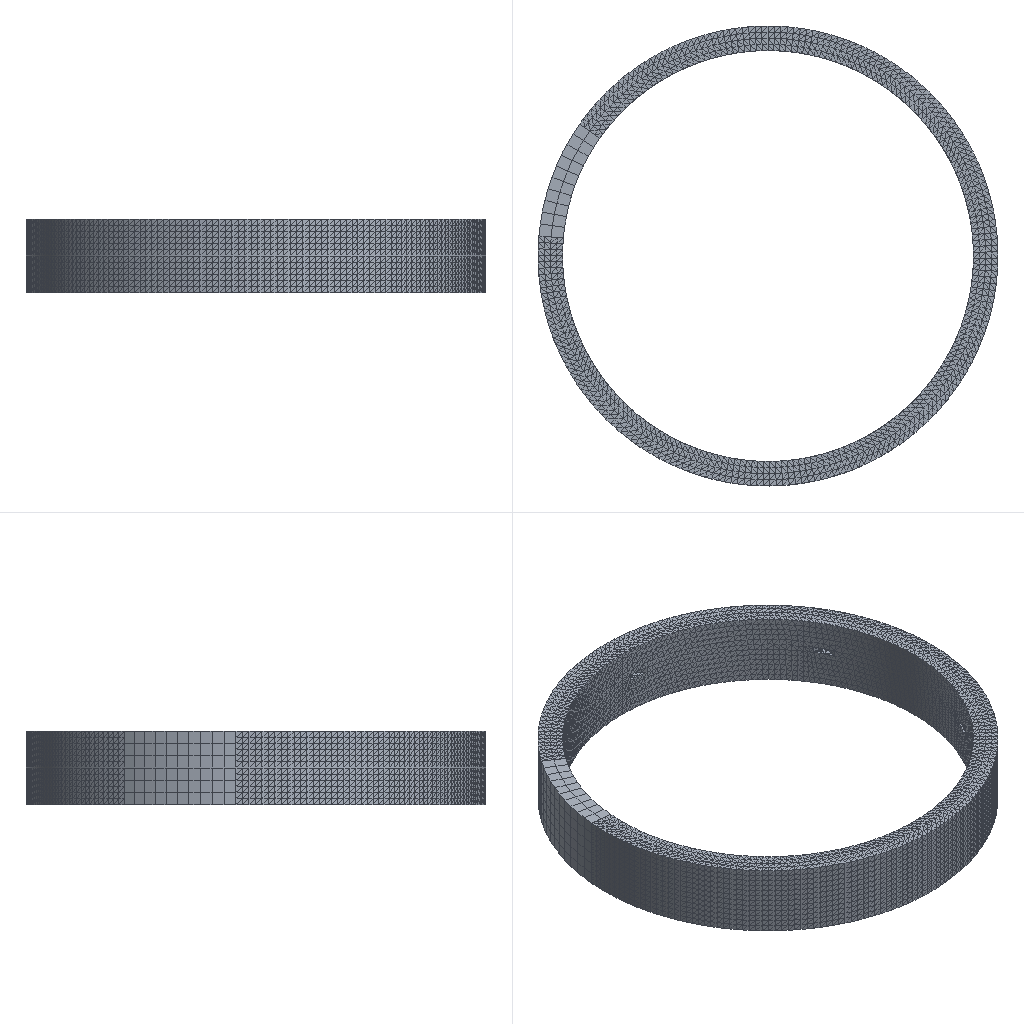Simulation study | abaqus
Set-up summary:
category,name,step,type,value,unit,region
solver,abaqus
solver,version,,,Abaqus/Standard 2020
units,not stated in the deck,,not stated
analysis,deck,,static,static
load_step,Step-1,Step-1,static
load_step,requested,,,1
mesh,nodes,,,120599
mesh,elements,,,97952
element_type,C3D4,,solid,24332
element_type,C3D10,,solid,73500
element_type,C3D8R,,solid,120
load,load commands in deck,,count,2
bc,support commands in deck,,count,1
material,GUANPIAN,,in results
material,LUOSHUAN,,in results
check,setup vs results,,match,"per instance, exact: element labels, types and connectivity; labels of the nodes the elements use; coordinates not compared"
Abaqus input file, long lists of numbers shortened, first 334 of 1919 lines:
*Heading
** Job name: Job-1 Model name: Model-1
** Generated by: Abaqus/CAE 2020
*Preprint, echo=NO, model=NO, history=NO, contact=NO
**
** PARTS
**
*Part, name=Part-1
*Node
      1,   5415.547,    6910.075,         600.
      2,   2137.132,    6910.075,         600.
** (18888 more lines like these left out)
*Element, type=C3D10
   1, 1664,  747, 1665, 1666, 2706, 2705, 2704, 2708, 2707, 2709
   2, 1667, 1666, 1665,  531, 2711, 2709, 2710, 2713, 2712, 2714
** (12248 more lines like these left out)
*Nset, nset=Set-33, generate
     1,  18890,      1
*Elset, elset=Set-33, generate
     1,  12250,      1
** Section: Section-1
*Solid Section, elset=Set-33, material=guanpian
,
*End Part
**
*Part, name=huan
*Node
      1,        -737.,   3267.925,        1200.
      2,  -907.02,   3224.875,        1200.
** (229 more lines like these left out)
*Element, type=C3D8R
  1,  78,  79,  90,  89,   1,   2,  13,  12
  2,  79,  80,  91,  90,   2,   3,  14,  13
** (118 more lines like these left out)
*Nset, nset=Set-1, generate
   1,  231,    1
*Elset, elset=Set-1, generate
   1,  120,    1
** Section: Section-1
*Solid Section, elset=Set-1, material=guanpian
,
*End Part
**
*Part, name=luoshuan
*Node
      1,   1815.458,  -103.665,   603.43
      2,   1794.725,  -75.309,    565.088
** (1002 more lines like these left out)
*Element, type=C3D4
  1, 842, 843, 844, 845
  2, 842, 846,  47,   7
** (3474 more lines like these left out)
*Nset, nset=Set-3, generate
    1,  1004,     1
*Elset, elset=Set-3, generate
    1,  3476,     1
** Section: Section-2
*Solid Section, elset=Set-3, material=luoshuan
,
*End Part
**
**
** ASSEMBLY
**
*Assembly, name=Assembly
**
*Instance, name=luoshuan-1, part=luoshuan
2639.383, 121.344, -1266.961
2639.383, 121.344, -1266.961, 2640.007, 121.614, -1266.228, 146.146
*End Instance
**
*Instance, name=Part-1-2, part=Part-1
4357.09, -7001.414,         600.
4357.09, -7001.414,         600., 4357.328, -7000.443,         600.,         180.
*End Instance
**
*Instance, name=luoshuan-1-rad-2, part=luoshuan
4357.446, -663.937, -1266.961
4357.446, -663.937, -1266.961, 4358.245, -663.994, -1266.362, 108.805
*End Instance
**
*Instance, name=luoshuan-1-rad-3, part=luoshuan
4699.623, -2521.711, -1266.961
4699.623, -2521.711, -1266.961, 4700.449, -2522.219, -1266.717, 84.284
*End Instance
**
*Instance, name=luoshuan-1-rad-4, part=luoshuan
3374.088, -3867.581, -1266.961
3374.088, -3867.581, -1266.961, 3374.579, -3868.402, -1267.251, 85.669
*End Instance
**
*Instance, name=Part-1-2-rad-2, part=Part-1
-491.939, -6156.447,         600.
-491.939, -6156.447,         600., -491.28, -6155.695,         600.,         180.
*End Instance
**
*Instance, name=Part-1-2-rad-3, part=Part-1
-2581.071, -1699.701,         600.
-2581.071, -1699.701,         600., -2580.139, -1699.339,         600.,         180.
*End Instance
**
*Instance, name=Part-1-2-rad-4, part=Part-1
-128.596, 2567.9,         600.
-128.596, 2567.9,         600., -127.602, 2567.791,         600.,         180.
*End Instance
**
*Instance, name=luoshuan-1-rad-2-1, part=luoshuan
1010.677, -835.593, -1266.961
1010.677, -835.593, -1266.961, 1011.089, -835.087, -1266.203, 187.52
*End Instance
**
*Instance, name=luoshuan-1-rad-3-1, part=luoshuan
698.5, -1799.706, -1266.961
698.5, -1799.706, -1266.961, 698.765, -1799.084, -1266.225, 211.514
*End Instance
**
*Instance, name=Part-1-2-rad-2-1, part=Part-1
7830.536, -3513.975,         600.
7830.536, -3513.975,         600., 7830.298, -3513.004,         600.,         180.
*End Instance
**
*Instance, name=luoshuan-1-rad-3-1-rad-2, part=luoshuan
1511.32, -3553.725, -1266.961
1511.32, -3553.725, -1266.961, 1511.366, -3554.509, -1267.581, 111.965
*End Instance
**
*Instance, name=Part-1-2-rad-3-1-rad-2, part=Part-1
4773.9, 3006.745,         600.
4773.9, 3006.745,         600., 4774.732, 3006.19,         600.,         180.
*End Instance
**
*Instance, name=huan-1, part=huan
2744.211, -1920.892,        -600.
2744.211, -1920.892,        -600., 2744.211, -1920.892, -599., 42.3
*End Instance
**
*Node
      1,   2744.159,  -1921.481,           0.
*Nset, nset=Set-5, instance=Part-1-2
     1,     4,     7,     8,    27,    28,    29,    30,   104,   105,   106,   107,   108,   149,   150,   151
   152,   153,   154,   155,   294,   300,   301,   302,   303,   304,   305,   306,   307,   308,   309,   310
** (24 more lines like these left out)
*Nset, nset=Set-5, instance=Part-1-2-rad-2
     1,     4,     7,     8,    27,    28,    29,    30,   104,   105,   106,   107,   108,   149,   150,   151
   152,   153,   154,   155,   294,   300,   301,   302,   303,   304,   305,   306,   307,   308,   309,   310
** (24 more lines like these left out)
*Nset, nset=Set-5, instance=Part-1-2-rad-3
     1,     4,     7,     8,    27,    28,    29,    30,   104,   105,   106,   107,   108,   149,   150,   151
   152,   153,   154,   155,   294,   300,   301,   302,   303,   304,   305,   306,   307,   308,   309,   310
** (24 more lines like these left out)
*Nset, nset=Set-5, instance=Part-1-2-rad-2-1
     1,     4,     7,     8,    27,    28,    29,    30,   104,   105,   106,   107,   108,   149,   150,   151
   152,   153,   154,   155,   294,   300,   301,   302,   303,   304,   305,   306,   307,   308,   309,   310
** (24 more lines like these left out)
*Nset, nset=Set-5, instance=Part-1-2-rad-4
     1,     4,     7,     8,    27,    28,    29,    30,   104,   105,   106,   107,   108,   149,   150,   151
   152,   153,   154,   155,   294,   300,   301,   302,   303,   304,   305,   306,   307,   308,   309,   310
** (24 more lines like these left out)
*Nset, nset=Set-5, instance=huan-1
  67,  68,  69,  70,  71,  72,  73,  74,  75,  76,  77, 144, 145, 146, 147, 148
 149, 150, 151, 152, 153, 154, 221, 222, 223, 224, 225, 226, 227, 228, 229, 230
** (1 more lines like these left out)
*Nset, nset=Set-5, instance=Part-1-2-rad-3-1-rad-2
     1,     4,     7,     8,    27,    28,    29,    30,   104,   105,   106,   107,   108,   149,   150,   151
   152,   153,   154,   155,   294,   300,   301,   302,   303,   304,   305,   306,   307,   308,   309,   310
** (24 more lines like these left out)
*Elset, elset=Set-5, instance=Part-1-2
  558,  646,  843, 1385, 1387, 1492, 1602, 1660, 1726, 1870, 2208, 2224, 2319, 2323, 2374, 2393
 2559, 2567, 2753, 2761, 2774, 2784, 2785, 2788, 6117, 6127, 6128, 6132, 6134, 6177, 6178, 6181
** (8 more lines like these left out)
*Elset, elset=Set-5, instance=Part-1-2-rad-2
  558,  646,  843, 1385, 1387, 1492, 1602, 1660, 1726, 1870, 2208, 2224, 2319, 2323, 2374, 2393
 2559, 2567, 2753, 2761, 2774, 2784, 2785, 2788, 6117, 6127, 6128, 6132, 6134, 6177, 6178, 6181
** (8 more lines like these left out)
*Elset, elset=Set-5, instance=Part-1-2-rad-3
  558,  646,  843, 1385, 1387, 1492, 1602, 1660, 1726, 1870, 2208, 2224, 2319, 2323, 2374, 2393
 2559, 2567, 2753, 2761, 2774, 2784, 2785, 2788, 6117, 6127, 6128, 6132, 6134, 6177, 6178, 6181
** (8 more lines like these left out)
*Elset, elset=Set-5, instance=Part-1-2-rad-2-1
  558,  646,  843, 1385, 1387, 1492, 1602, 1660, 1726, 1870, 2208, 2224, 2319, 2323, 2374, 2393
 2559, 2567, 2753, 2761, 2774, 2784, 2785, 2788, 6117, 6127, 6128, 6132, 6134, 6177, 6178, 6181
** (8 more lines like these left out)
*Elset, elset=Set-5, instance=Part-1-2-rad-4
  558,  646,  843, 1385, 1387, 1492, 1602, 1660, 1726, 1870, 2208, 2224, 2319, 2323, 2374, 2393
 2559, 2567, 2753, 2761, 2774, 2784, 2785, 2788, 6117, 6127, 6128, 6132, 6134, 6177, 6178, 6181
** (8 more lines like these left out)
*Elset, elset=Set-5, instance=huan-1
  51,  52,  53,  54,  55,  56,  57,  58,  59,  60, 111, 112, 113, 114, 115, 116
 117, 118, 119, 120
*Elset, elset=Set-5, instance=Part-1-2-rad-3-1-rad-2
  558,  646,  843, 1385, 1387, 1492, 1602, 1660, 1726, 1870, 2208, 2224, 2319, 2323, 2374, 2393
 2559, 2567, 2753, 2761, 2774, 2784, 2785, 2788, 6117, 6127, 6128, 6132, 6134, 6177, 6178, 6181
** (8 more lines like these left out)
*Nset, nset=Set-7
 1,
*Nset, nset=Set-8
 1,
*Nset, nset=Set-9, instance=Part-1-2
     1,     4,     7,     8,    27,    28,    29,    30,   104,   105,   106,   107,   108,   149,   150,   151
   152,   153,   154,   155,   294,   300,   301,   302,   303,   304,   305,   306,   307,   308,   309,   310
** (24 more lines like these left out)
*Nset, nset=Set-9, instance=Part-1-2-rad-2
     1,     4,     7,     8,    27,    28,    29,    30,   104,   105,   106,   107,   108,   149,   150,   151
   152,   153,   154,   155,   294,   300,   301,   302,   303,   304,   305,   306,   307,   308,   309,   310
** (24 more lines like these left out)
*Nset, nset=Set-9, instance=Part-1-2-rad-3
     1,     4,     7,     8,    27,    28,    29,    30,   104,   105,   106,   107,   108,   149,   150,   151
   152,   153,   154,   155,   294,   300,   301,   302,   303,   304,   305,   306,   307,   308,   309,   310
** (24 more lines like these left out)
*Nset, nset=Set-9, instance=Part-1-2-rad-2-1
     1,     4,     7,     8,    27,    28,    29,    30,   104,   105,   106,   107,   108,   149,   150,   151
   152,   153,   154,   155,   294,   300,   301,   302,   303,   304,   305,   306,   307,   308,   309,   310
** (24 more lines like these left out)
*Nset, nset=Set-9, instance=Part-1-2-rad-4
     1,     4,     7,     8,    27,    28,    29,    30,   104,   105,   106,   107,   108,   149,   150,   151
   152,   153,   154,   155,   294,   300,   301,   302,   303,   304,   305,   306,   307,   308,   309,   310
** (24 more lines like these left out)
*Nset, nset=Set-9, instance=Part-1-2-rad-3-1-rad-2
     1,     4,     7,     8,    27,    28,    29,    30,   104,   105,   106,   107,   108,   149,   150,   151
   152,   153,   154,   155,   294,   300,   301,   302,   303,   304,   305,   306,   307,   308,   309,   310
** (24 more lines like these left out)
*Elset, elset=Set-9, instance=Part-1-2
  558,  646,  843, 1385, 1387, 1492, 1602, 1660, 1726, 1870, 2208, 2224, 2319, 2323, 2374, 2393
 2559, 2567, 2753, 2761, 2774, 2784, 2785, 2788, 6117, 6127, 6128, 6132, 6134, 6177, 6178, 6181
** (8 more lines like these left out)
*Elset, elset=Set-9, instance=Part-1-2-rad-2
  558,  646,  843, 1385, 1387, 1492, 1602, 1660, 1726, 1870, 2208, 2224, 2319, 2323, 2374, 2393
 2559, 2567, 2753, 2761, 2774, 2784, 2785, 2788, 6117, 6127, 6128, 6132, 6134, 6177, 6178, 6181
** (8 more lines like these left out)
*Elset, elset=Set-9, instance=Part-1-2-rad-3
  558,  646,  843, 1385, 1387, 1492, 1602, 1660, 1726, 1870, 2208, 2224, 2319, 2323, 2374, 2393
 2559, 2567, 2753, 2761, 2774, 2784, 2785, 2788, 6117, 6127, 6128, 6132, 6134, 6177, 6178, 6181
** (8 more lines like these left out)
*Elset, elset=Set-9, instance=Part-1-2-rad-2-1
  558,  646,  843, 1385, 1387, 1492, 1602, 1660, 1726, 1870, 2208, 2224, 2319, 2323, 2374, 2393
 2559, 2567, 2753, 2761, 2774, 2784, 2785, 2788, 6117, 6127, 6128, 6132, 6134, 6177, 6178, 6181
** (8 more lines like these left out)
*Elset, elset=Set-9, instance=Part-1-2-rad-4
  558,  646,  843, 1385, 1387, 1492, 1602, 1660, 1726, 1870, 2208, 2224, 2319, 2323, 2374, 2393
 2559, 2567, 2753, 2761, 2774, 2784, 2785, 2788, 6117, 6127, 6128, 6132, 6134, 6177, 6178, 6181
** (8 more lines like these left out)
*Elset, elset=Set-9, instance=Part-1-2-rad-3-1-rad-2
  558,  646,  843, 1385, 1387, 1492, 1602, 1660, 1726, 1870, 2208, 2224, 2319, 2323, 2374, 2393
 2559, 2567, 2753, 2761, 2774, 2784, 2785, 2788, 6117, 6127, 6128, 6132, 6134, 6177, 6178, 6181
** (8 more lines like these left out)
*Nset, nset=m_Set-6, instance=luoshuan-1, generate
    1,  1004,     1
*Nset, nset=m_Set-6, instance=luoshuan-1-rad-2, generate
    1,  1004,     1
*Nset, nset=m_Set-6, instance=luoshuan-1-rad-4, generate
    1,  1004,     1
*Nset, nset=m_Set-6, instance=luoshuan-1-rad-2-1, generate
    1,  1004,     1
*Nset, nset=m_Set-6, instance=luoshuan-1-rad-3-1-rad-2, generate
    1,  1004,     1
*Nset, nset=m_Set-6, instance=luoshuan-1-rad-3, generate
    1,  1004,     1
*Nset, nset=m_Set-6, instance=luoshuan-1-rad-3-1, generate
    1,  1004,     1
*Elset, elset=m_Set-6, instance=luoshuan-1, generate
    1,  3476,     1
*Elset, elset=m_Set-6, instance=luoshuan-1-rad-2, generate
    1,  3476,     1
*Elset, elset=m_Set-6, instance=luoshuan-1-rad-4, generate
    1,  3476,     1
*Elset, elset=m_Set-6, instance=luoshuan-1-rad-2-1, generate
    1,  3476,     1
*Elset, elset=m_Set-6, instance=luoshuan-1-rad-3-1-rad-2, generate
    1,  3476,     1
*Elset, elset=m_Set-6, instance=luoshuan-1-rad-3, generate
    1,  3476,     1
*Elset, elset=m_Set-6, instance=luoshuan-1-rad-3-1, generate
    1,  3476,     1
*Nset, nset=m_Set-8
 1,
*Nset, nset=view, instance=Part-1-2
     1,     2,     3,     4,     5,     6,     7,     8,     9,    10,    11,    12,    13,    14,    15,    16
    17,    18,    19,    20,    21,    22,    23,    24,    25,    26,    33,    34,    35,    36,    37,    38
** (605 more lines like these left out)
*Elset, elset=view, instance=Part-1-2, generate
    1,  6064,     1
*Elset, elset=_guanbi2_S3, internal, instance=Part-1-2
    13,    38,    52,    57,    59,    62,    76,    99,   108,   134,   141,   171,   199,   208,   223,   231
   260,   303,   310,   327,   328,   331,   341,   356,   358,   369,   375,   447,   452,   455,   483,   485
** (18 more lines like these left out)
*Elset, elset=_guanbi2_S4, internal, instance=Part-1-2
   872,  1332,  1636,  1699,  1718,  8265,  8565,  9861, 11578, 11587, 11635, 11995
*Elset, elset=_guanbi2_S1, internal, instance=Part-1-2
  1567,  1573,  1660,  2679,  2870,  3007,  9637, 11792, 12007, 12142
*Elset, elset=_guanbi2_S2, internal, instance=Part-1-2
   634,  1587,  1589,  1628, 10122, 11606
*Surface, type=ELEMENT, name=guanbi2
_guanbi2_S3, S3
_guanbi2_S4, S4
_guanbi2_S2, S2
_guanbi2_S1, S1
*Elset, elset=_luokong_S4, internal, instance=Part-1-2
 4401, 6020, 6056, 6057
*Elset, elset=_luokong_S3, internal, instance=Part-1-2
 4545, 5042, 5501
*Elset, elset=_luokong_S2, internal, instance=Part-1-2
 5043, 6060
*Elset, elset=_luokong_S1, internal, instance=Part-1-2
 5278, 5449, 5955
*Surface, type=ELEMENT, name=luokong
_luokong_S4, S4
_luokong_S3, S3
_luokong_S2, S2
_luokong_S1, S1
*Elset, elset=_luomao1_S3, internal, instance=luoshuan-1
  148,  151,  190,  193,  317,  318,  320,  321,  328,  554,  820,  823,  830,  836,  840, 2630
 2636, 2695, 2697, 2844, 2858, 2859, 2943, 2945, 2955, 2966, 3361, 3408, 3437, 3442, 3443, 3445
** (1 more lines like these left out)
*Elset, elset=_luomao1_S4, internal, instance=luoshuan-1
  150,  694, 2783, 3454
*Elset, elset=_luomao1_S2, internal, instance=luoshuan-1
 335,
*Surface, type=ELEMENT, name=luomao1
_luomao1_S3, S3
_luomao1_S4, S4
_luomao1_S2, S2
*Elset, elset=_luomao2_S3, internal, instance=luoshuan-1
  946,  998, 1056, 1074, 1078, 1082, 1179, 1180, 1489, 1509, 1549, 1663, 1697, 1703, 1744, 1759
 1787, 1875, 1887, 1889, 1981, 2078, 2079, 2479, 2487, 2491, 2494, 2497, 2504, 2519, 2522
*Elset, elset=_luomao2_S4, internal, instance=luoshuan-1
 1387, 1694, 2495, 2521
*Elset, elset=_luomao2_S2, internal, instance=luoshuan-1
 1698,
*Surface, type=ELEMENT, name=luomao2
_luomao2_S3, S3
_luomao2_S4, S4
_luomao2_S2, S2
*Elset, elset=_luoshuan_S2, internal, instance=luoshuan-1
    8,   85,   96,  189,  233,  244,  278,  373,  472,  482,  487,  492,  497,  505,  508,  509
Last 516 lines:
*Elset, elset=__Int-1_gcs0_226_S2, internal, instance=luoshuan-1-rad-2-1
  858, 1098, 1191, 1193, 1234, 1250, 1357, 1361, 1363, 1368, 1374, 1375, 1383, 1384, 1390, 1403
 1407, 1412, 1418, 1425, 1430, 1441, 1443, 1449, 1450, 1452, 1455, 1457, 1460, 1463, 1468, 1475
** (3 more lines like these left out)
*Elset, elset=__Int-1_gcs0_226_S1, internal, instance=luoshuan-1-rad-2-1
  876,  909,  992, 1025, 1026, 1089, 1157, 1194, 1197, 1200, 1204, 1237, 1245, 1253, 1265, 1267
 1268, 1285, 1300, 1306, 1309, 1315, 1318, 1326, 1339, 1347, 1358, 1369, 1378, 1382, 1389, 1391
** (3 more lines like these left out)
*Elset, elset=__Int-1_gcs0_226_S3, internal, instance=luoshuan-1-rad-2-1
  898,  905,  908,  927,  930,  961, 1140, 1141, 1156, 1158, 1164, 1169, 1173, 1185, 1195, 1199
 1202, 1205, 1209, 1211, 1212, 1216, 1219, 1221, 1222, 1223, 1226, 1227, 1228, 1230, 1232, 1236
** (6 more lines like these left out)
*Elset, elset=__Int-1_gcs0_226_S4, internal, instance=luoshuan-1-rad-2-1
 1304, 1510, 1704, 1705
*Surface, type=ELEMENT, name=_Int-1_gcs0_226, internal
__Int-1_gcs0_226_S2, S2
__Int-1_gcs0_226_S1, S1
__Int-1_gcs0_226_S4, S4
__Int-1_gcs0_226_S3, S3
*Elset, elset=__Int-1_gcs0_229_S3, internal, instance=luoshuan-1-rad-2-1
 2656, 2657, 2759, 2760, 2769, 2775, 2821, 2824, 2975, 3038, 3090, 3148, 3209, 3210, 3242, 3247
 3259, 3277, 3300, 3301, 3355, 3365, 3369, 3372, 3376, 3419, 3422, 3423, 3452, 3473, 3475
*Elset, elset=__Int-1_gcs0_229_S4, internal, instance=luoshuan-1-rad-2-1
 2840,
*Surface, type=ELEMENT, name=_Int-1_gcs0_229, internal
__Int-1_gcs0_229_S3, S3
__Int-1_gcs0_229_S4, S4
*Elset, elset=__Int-1_gcs0_231_S1, internal, instance=luoshuan-1-rad-2-1
 2704, 2745, 2876, 2877, 2937, 2980, 2985, 2988, 3055, 3067, 3081, 3083, 3092, 3094, 3099, 3157
 3163, 3165, 3190, 3191, 3205, 3214, 3215, 3220, 3222, 3223, 3225, 3232, 3236, 3257, 3262, 3266
** (2 more lines like these left out)
*Elset, elset=__Int-1_gcs0_231_S2, internal, instance=luoshuan-1-rad-2-1
 2728, 2735, 2940, 2983, 3140, 3216, 3219, 3230, 3231, 3240, 3248, 3254, 3261, 3264, 3268, 3269
 3275, 3276, 3279, 3280, 3283, 3285, 3287, 3296, 3297, 3299, 3303, 3304, 3315, 3318, 3320, 3322
** (2 more lines like these left out)
*Elset, elset=__Int-1_gcs0_231_S3, internal, instance=luoshuan-1-rad-2-1
 2742, 2744, 2761, 2780, 2804, 2807, 2875, 2898, 2902, 2905, 2913, 2920, 2925, 2938, 2939, 2941
 2947, 2969, 2970, 2971, 2976, 2977, 2978, 2979, 2982, 2984, 2986, 2987, 2990, 2991, 2994, 2995
** (9 more lines like these left out)
*Elset, elset=__Int-1_gcs0_231_S4, internal, instance=luoshuan-1-rad-2-1
 2874, 2899, 2942, 3306
*Surface, type=ELEMENT, name=_Int-1_gcs0_231, internal
__Int-1_gcs0_231_S1, S1
__Int-1_gcs0_231_S2, S2
__Int-1_gcs0_231_S4, S4
__Int-1_gcs0_231_S3, S3
*Elset, elset=__Int-1_gcs0_235_S2, internal, instance=luoshuan-1-rad-3-1
   8,  85,  96, 189, 233, 244, 278, 373, 472, 482, 487, 492, 497, 505, 508, 509
 512, 518, 524, 529, 536, 540, 547, 584, 590, 596, 599, 602, 606, 608, 610, 613
** (4 more lines like these left out)
*Elset, elset=__Int-1_gcs0_235_S3, internal, instance=luoshuan-1-rad-3-1
  21, 122, 131, 142, 226, 230, 271, 272, 273, 286, 290, 291, 300, 303, 307, 311
 313, 315, 337, 342, 343, 347, 349, 353, 354, 359, 360, 362, 366, 367, 369, 375
** (6 more lines like these left out)
*Elset, elset=__Int-1_gcs0_235_S1, internal, instance=luoshuan-1-rad-3-1
 110, 125, 177, 294, 344, 348, 350, 351, 363, 385, 386, 388, 393, 395, 404, 431
 434, 439, 457, 491, 498, 501, 513, 550, 551, 570, 583, 585, 592, 595, 597, 598
** (3 more lines like these left out)
*Elset, elset=__Int-1_gcs0_235_S4, internal, instance=luoshuan-1-rad-3-1
 225, 252, 355, 537, 636, 680, 704, 723, 767, 777
*Surface, type=ELEMENT, name=_Int-1_gcs0_235, internal
__Int-1_gcs0_235_S2, S2
__Int-1_gcs0_235_S3, S3
__Int-1_gcs0_235_S4, S4
__Int-1_gcs0_235_S1, S1
*Elset, elset=__Int-1_gcs0_237_S3, internal, instance=luoshuan-1-rad-3-1
  29,  37, 132, 162, 168, 194, 444, 462, 484, 489, 544, 548, 552, 576, 587, 600
 607, 615, 620, 642, 651, 660, 671, 683, 728, 743, 752, 764, 804
*Elset, elset=__Int-1_gcs0_237_S2, internal, instance=luoshuan-1-rad-3-1
 135, 694, 699
*Surface, type=ELEMENT, name=_Int-1_gcs0_237, internal
__Int-1_gcs0_237_S3, S3
__Int-1_gcs0_237_S2, S2
*Elset, elset=__Int-1_gcs0_243_S3, internal, instance=luoshuan-1-rad-3-1
  866,  868, 1043, 1044, 1050, 1052, 1053, 1102, 1104, 1187, 1297, 1325, 1371, 1387, 1398, 1404
 1433, 1435, 1454, 1470, 1476, 1479, 1486, 1488, 1517, 1526, 1561, 1562, 1573, 1598, 1695, 1709
*Surface, type=ELEMENT, name=_Int-1_gcs0_243, internal
__Int-1_gcs0_243_S3, S3
*Elset, elset=__Int-1_gcs0_244_S3, internal, instance=luoshuan-1-rad-3-1
 1806, 1867, 1915, 1916, 1917, 1927, 1932, 2009, 2020, 2022, 2026, 2029, 2036, 2040, 2050, 2056
 2062, 2063, 2064, 2065, 2075, 2088, 2089, 2091, 2094, 2098, 2100, 2104, 2106, 2108, 2110, 2112
** (15 more lines like these left out)
*Elset, elset=__Int-1_gcs0_244_S4, internal, instance=luoshuan-1-rad-3-1
 1921, 2220, 2247
*Elset, elset=__Int-1_gcs0_244_S1, internal, instance=luoshuan-1-rad-3-1
 2157, 2451, 2459, 2477, 2536
*Elset, elset=__Int-1_gcs0_244_S2, internal, instance=luoshuan-1-rad-3-1
 2474,
*Surface, type=ELEMENT, name=_Int-1_gcs0_244, internal
__Int-1_gcs0_244_S3, S3
__Int-1_gcs0_244_S4, S4
__Int-1_gcs0_244_S2, S2
__Int-1_gcs0_244_S1, S1
*Elset, elset=__Int-1_gcs0_248_S3, internal, instance=luoshuan-1-rad-3-1
 1763, 1764, 1765, 1834, 1908, 1934, 1937, 1939, 2080, 2083, 2193, 2472, 2480, 2483, 2512, 2517
 2529, 2530, 2535, 2539, 2549, 2552, 2557, 2559, 2560, 2561, 2576, 2580, 2582, 2585, 2594
*Elset, elset=__Int-1_gcs0_248_S4, internal, instance=luoshuan-1-rad-3-1
 2569,
*Surface, type=ELEMENT, name=_Int-1_gcs0_248, internal
__Int-1_gcs0_248_S3, S3
__Int-1_gcs0_248_S4, S4
*Elset, elset=__Int-1_gcs0_250_S2, internal, instance=luoshuan-1-rad-3-1
  858, 1098, 1191, 1193, 1234, 1250, 1357, 1361, 1363, 1368, 1374, 1375, 1383, 1384, 1390, 1403
 1407, 1412, 1418, 1425, 1430, 1441, 1443, 1449, 1450, 1452, 1455, 1457, 1460, 1463, 1468, 1475
** (3 more lines like these left out)
*Elset, elset=__Int-1_gcs0_250_S1, internal, instance=luoshuan-1-rad-3-1
  876,  909,  992, 1025, 1026, 1089, 1157, 1194, 1197, 1200, 1204, 1237, 1245, 1253, 1265, 1267
 1268, 1285, 1300, 1306, 1309, 1315, 1318, 1326, 1339, 1347, 1358, 1369, 1378, 1382, 1389, 1391
** (3 more lines like these left out)
*Elset, elset=__Int-1_gcs0_250_S3, internal, instance=luoshuan-1-rad-3-1
  898,  905,  908,  927,  930,  961, 1140, 1141, 1156, 1158, 1164, 1169, 1173, 1185, 1195, 1199
 1202, 1205, 1209, 1211, 1212, 1216, 1219, 1221, 1222, 1223, 1226, 1227, 1228, 1230, 1232, 1236
** (6 more lines like these left out)
*Elset, elset=__Int-1_gcs0_250_S4, internal, instance=luoshuan-1-rad-3-1
 1304, 1510, 1704, 1705
*Surface, type=ELEMENT, name=_Int-1_gcs0_250, internal
__Int-1_gcs0_250_S2, S2
__Int-1_gcs0_250_S1, S1
__Int-1_gcs0_250_S4, S4
__Int-1_gcs0_250_S3, S3
*Elset, elset=__Int-1_gcs0_253_S3, internal, instance=luoshuan-1-rad-3-1
 2656, 2657, 2759, 2760, 2769, 2775, 2821, 2824, 2975, 3038, 3090, 3148, 3209, 3210, 3242, 3247
 3259, 3277, 3300, 3301, 3355, 3365, 3369, 3372, 3376, 3419, 3422, 3423, 3452, 3473, 3475
*Elset, elset=__Int-1_gcs0_253_S4, internal, instance=luoshuan-1-rad-3-1
 2840,
*Surface, type=ELEMENT, name=_Int-1_gcs0_253, internal
__Int-1_gcs0_253_S3, S3
__Int-1_gcs0_253_S4, S4
*Elset, elset=__Int-1_gcs0_255_S1, internal, instance=luoshuan-1-rad-3-1
 2704, 2745, 2876, 2877, 2937, 2980, 2985, 2988, 3055, 3067, 3081, 3083, 3092, 3094, 3099, 3157
 3163, 3165, 3190, 3191, 3205, 3214, 3215, 3220, 3222, 3223, 3225, 3232, 3236, 3257, 3262, 3266
** (2 more lines like these left out)
*Elset, elset=__Int-1_gcs0_255_S2, internal, instance=luoshuan-1-rad-3-1
 2728, 2735, 2940, 2983, 3140, 3216, 3219, 3230, 3231, 3240, 3248, 3254, 3261, 3264, 3268, 3269
 3275, 3276, 3279, 3280, 3283, 3285, 3287, 3296, 3297, 3299, 3303, 3304, 3315, 3318, 3320, 3322
** (2 more lines like these left out)
*Elset, elset=__Int-1_gcs0_255_S3, internal, instance=luoshuan-1-rad-3-1
 2742, 2744, 2761, 2780, 2804, 2807, 2875, 2898, 2902, 2905, 2913, 2920, 2925, 2938, 2939, 2941
 2947, 2969, 2970, 2971, 2976, 2977, 2978, 2979, 2982, 2984, 2986, 2987, 2990, 2991, 2994, 2995
** (9 more lines like these left out)
*Elset, elset=__Int-1_gcs0_255_S4, internal, instance=luoshuan-1-rad-3-1
 2874, 2899, 2942, 3306
*Surface, type=ELEMENT, name=_Int-1_gcs0_255, internal
__Int-1_gcs0_255_S1, S1
__Int-1_gcs0_255_S2, S2
__Int-1_gcs0_255_S4, S4
__Int-1_gcs0_255_S3, S3
*Elset, elset=__Int-1_gcs0_266_S3, internal, instance=Part-1-2-rad-2-1
 3642, 6048
*Elset, elset=__Int-1_gcs0_266_S2, internal, instance=Part-1-2-rad-2-1
 3789, 4502
*Elset, elset=__Int-1_gcs0_266_S4, internal, instance=Part-1-2-rad-2-1
 4743,
*Elset, elset=__Int-1_gcs0_266_S1, internal, instance=Part-1-2-rad-2-1
 6051,
*Surface, type=ELEMENT, name=_Int-1_gcs0_266, internal
__Int-1_gcs0_266_S3, S3
__Int-1_gcs0_266_S2, S2
__Int-1_gcs0_266_S4, S4
__Int-1_gcs0_266_S1, S1
*Elset, elset=__Int-1_gcs0_275_S4, internal, instance=Part-1-2-rad-2-1
 3113, 4505, 4652, 4754, 5023, 5211, 5239, 5339, 5390, 5508, 5552, 6039
*Elset, elset=__Int-1_gcs0_275_S3, internal, instance=Part-1-2-rad-2-1
 3130, 3134, 3152, 3157, 3188, 3189, 3192, 3206, 3211, 3212, 3216, 3218, 3236, 3254, 3267, 3294
 3317, 3324, 3327, 3336, 3340, 3349, 3363, 3365, 3366, 3377, 3384, 3389, 3390, 3401, 3402, 3408
** (19 more lines like these left out)
*Elset, elset=__Int-1_gcs0_275_S1, internal, instance=Part-1-2-rad-2-1
 3142, 3163, 4197, 4282, 5079, 5326, 5327, 5609, 5648, 5657, 5757, 5973
*Elset, elset=__Int-1_gcs0_275_S2, internal, instance=Part-1-2-rad-2-1
 4680, 4696, 4856, 4961, 5036, 5050, 5070, 5244, 5255, 5259, 5262, 5308, 5323, 5355, 5393, 5401
 5618, 5652, 5756, 5777, 5798, 5848, 6003
*Surface, type=ELEMENT, name=_Int-1_gcs0_275, internal
__Int-1_gcs0_275_S4, S4
__Int-1_gcs0_275_S3, S3
__Int-1_gcs0_275_S2, S2
__Int-1_gcs0_275_S1, S1
*Elset, elset=__Int-1_gcs0_277_S3, internal, instance=Part-1-2-rad-2-1
 6093, 6108, 6140, 6145, 6147, 6157, 6173, 6182, 6191, 6202, 6207, 6217, 6230, 6267, 6329, 6350
 6364, 6379, 6391, 6399, 6400, 6402, 6422, 6478, 6482, 6519, 6573, 6579, 6582, 6648, 6667, 6709
** (22 more lines like these left out)
*Elset, elset=__Int-1_gcs0_277_S2, internal, instance=Part-1-2-rad-2-1
 6167, 7776, 8152, 8319
*Elset, elset=__Int-1_gcs0_277_S4, internal, instance=Part-1-2-rad-2-1
 6177, 6971, 7617, 7693, 7725, 7747, 7753, 7754, 7879, 8119, 8327, 8402, 8790, 8829
*Elset, elset=__Int-1_gcs0_277_S1, internal, instance=Part-1-2-rad-2-1
 6278, 7028, 7767, 8334, 8432, 9146
*Surface, type=ELEMENT, name=_Int-1_gcs0_277, internal
__Int-1_gcs0_277_S3, S3
__Int-1_gcs0_277_S2, S2
__Int-1_gcs0_277_S4, S4
__Int-1_gcs0_277_S1, S1
*Elset, elset=__Int-1_gcs0_280_S3, internal, instance=Part-1-2-rad-2-1
   17,   37,   73,   87,   92,  112,  121,  129,  140,  142,  149,  155,  170,  183,  184,  191
  198,  220,  226,  230,  242,  247,  248,  251,  252,  277,  283,  290,  340,  352,  363,  413
** (22 more lines like these left out)
*Elset, elset=__Int-1_gcs0_280_S4, internal, instance=Part-1-2-rad-2-1
  152, 1289, 1501, 1546, 1645, 1751, 1757, 1770, 1815, 2912
*Elset, elset=__Int-1_gcs0_280_S1, internal, instance=Part-1-2-rad-2-1
  262,  472, 1841, 2812
*Elset, elset=__Int-1_gcs0_280_S2, internal, instance=Part-1-2-rad-2-1
  767, 1542, 1585, 1647, 1706, 1802, 1804, 1915, 1968, 2808
*Surface, type=ELEMENT, name=_Int-1_gcs0_280, internal
__Int-1_gcs0_280_S3, S3
__Int-1_gcs0_280_S4, S4
__Int-1_gcs0_280_S2, S2
__Int-1_gcs0_280_S1, S1
*Elset, elset=__Int-1_gcs0_282_S3, internal, instance=Part-1-2-rad-2-1
  9190,  9210,  9225,  9248,  9249,  9275,  9288,  9293,  9327,  9352,  9418,  9437,  9446,  9501,  9563,  9634
  9792,  9875, 10100, 10107, 10231, 10256, 10259, 10291, 10341, 10344, 10362, 10386, 10390, 10458, 10459, 10473
** (23 more lines like these left out)
*Elset, elset=__Int-1_gcs0_282_S1, internal, instance=Part-1-2-rad-2-1
  9222,  9250,  9292,  9322, 11350, 11517, 11646
*Elset, elset=__Int-1_gcs0_282_S4, internal, instance=Part-1-2-rad-2-1
  9270,  9567,  9709, 11416, 11431, 11449, 11639
*Elset, elset=__Int-1_gcs0_282_S2, internal, instance=Part-1-2-rad-2-1
 10732, 10948, 11071, 11201, 11354, 11388, 11398, 11461, 11525
*Surface, type=ELEMENT, name=_Int-1_gcs0_282, internal
__Int-1_gcs0_282_S3, S3
__Int-1_gcs0_282_S1, S1
__Int-1_gcs0_282_S4, S4
__Int-1_gcs0_282_S2, S2
*Elset, elset=__Int-1_gcs0_287_S2, internal, instance=luoshuan-1-rad-3-1-rad-2
   8,  85,  96, 189, 233, 244, 278, 373, 472, 482, 487, 492, 497, 505, 508, 509
 512, 518, 524, 529, 536, 540, 547, 584, 590, 596, 599, 602, 606, 608, 610, 613
** (4 more lines like these left out)
*Elset, elset=__Int-1_gcs0_287_S3, internal, instance=luoshuan-1-rad-3-1-rad-2
  21, 122, 131, 142, 226, 230, 271, 272, 273, 286, 290, 291, 300, 303, 307, 311
 313, 315, 337, 342, 343, 347, 349, 353, 354, 359, 360, 362, 366, 367, 369, 375
** (6 more lines like these left out)
*Elset, elset=__Int-1_gcs0_287_S1, internal, instance=luoshuan-1-rad-3-1-rad-2
 110, 125, 177, 294, 344, 348, 350, 351, 363, 385, 386, 388, 393, 395, 404, 431
 434, 439, 457, 491, 498, 501, 513, 550, 551, 570, 583, 585, 592, 595, 597, 598
** (3 more lines like these left out)
*Elset, elset=__Int-1_gcs0_287_S4, internal, instance=luoshuan-1-rad-3-1-rad-2
 225, 252, 355, 537, 636, 680, 704, 723, 767, 777
*Surface, type=ELEMENT, name=_Int-1_gcs0_287, internal
__Int-1_gcs0_287_S2, S2
__Int-1_gcs0_287_S3, S3
__Int-1_gcs0_287_S4, S4
__Int-1_gcs0_287_S1, S1
*Elset, elset=__Int-1_gcs0_289_S3, internal, instance=luoshuan-1-rad-3-1-rad-2
  29,  37, 132, 162, 168, 194, 444, 462, 484, 489, 544, 548, 552, 576, 587, 600
 607, 615, 620, 642, 651, 660, 671, 683, 728, 743, 752, 764, 804
*Elset, elset=__Int-1_gcs0_289_S2, internal, instance=luoshuan-1-rad-3-1-rad-2
 135, 694, 699
*Surface, type=ELEMENT, name=_Int-1_gcs0_289, internal
__Int-1_gcs0_289_S3, S3
__Int-1_gcs0_289_S2, S2
*Elset, elset=__Int-1_gcs0_295_S3, internal, instance=luoshuan-1-rad-3-1-rad-2
  866,  868, 1043, 1044, 1050, 1052, 1053, 1102, 1104, 1187, 1297, 1325, 1371, 1387, 1398, 1404
 1433, 1435, 1454, 1470, 1476, 1479, 1486, 1488, 1517, 1526, 1561, 1562, 1573, 1598, 1695, 1709
*Surface, type=ELEMENT, name=_Int-1_gcs0_295, internal
__Int-1_gcs0_295_S3, S3
*Elset, elset=__Int-1_gcs0_296_S3, internal, instance=luoshuan-1-rad-3-1-rad-2
 1806, 1867, 1915, 1916, 1917, 1927, 1932, 2009, 2020, 2022, 2026, 2029, 2036, 2040, 2050, 2056
 2062, 2063, 2064, 2065, 2075, 2088, 2089, 2091, 2094, 2098, 2100, 2104, 2106, 2108, 2110, 2112
** (15 more lines like these left out)
*Elset, elset=__Int-1_gcs0_296_S4, internal, instance=luoshuan-1-rad-3-1-rad-2
 1921, 2220, 2247
*Elset, elset=__Int-1_gcs0_296_S1, internal, instance=luoshuan-1-rad-3-1-rad-2
 2157, 2451, 2459, 2477, 2536
*Elset, elset=__Int-1_gcs0_296_S2, internal, instance=luoshuan-1-rad-3-1-rad-2
 2474,
*Surface, type=ELEMENT, name=_Int-1_gcs0_296, internal
__Int-1_gcs0_296_S3, S3
__Int-1_gcs0_296_S4, S4
__Int-1_gcs0_296_S2, S2
__Int-1_gcs0_296_S1, S1
*Elset, elset=__Int-1_gcs0_300_S3, internal, instance=luoshuan-1-rad-3-1-rad-2
 1763, 1764, 1765, 1834, 1908, 1934, 1937, 1939, 2080, 2083, 2193, 2472, 2480, 2483, 2512, 2517
 2529, 2530, 2535, 2539, 2549, 2552, 2557, 2559, 2560, 2561, 2576, 2580, 2582, 2585, 2594
*Elset, elset=__Int-1_gcs0_300_S4, internal, instance=luoshuan-1-rad-3-1-rad-2
 2569,
*Surface, type=ELEMENT, name=_Int-1_gcs0_300, internal
__Int-1_gcs0_300_S3, S3
__Int-1_gcs0_300_S4, S4
*Elset, elset=__Int-1_gcs0_302_S2, internal, instance=luoshuan-1-rad-3-1-rad-2
  858, 1098, 1191, 1193, 1234, 1250, 1357, 1361, 1363, 1368, 1374, 1375, 1383, 1384, 1390, 1403
 1407, 1412, 1418, 1425, 1430, 1441, 1443, 1449, 1450, 1452, 1455, 1457, 1460, 1463, 1468, 1475
** (3 more lines like these left out)
*Elset, elset=__Int-1_gcs0_302_S1, internal, instance=luoshuan-1-rad-3-1-rad-2
  876,  909,  992, 1025, 1026, 1089, 1157, 1194, 1197, 1200, 1204, 1237, 1245, 1253, 1265, 1267
 1268, 1285, 1300, 1306, 1309, 1315, 1318, 1326, 1339, 1347, 1358, 1369, 1378, 1382, 1389, 1391
** (3 more lines like these left out)
*Elset, elset=__Int-1_gcs0_302_S3, internal, instance=luoshuan-1-rad-3-1-rad-2
  898,  905,  908,  927,  930,  961, 1140, 1141, 1156, 1158, 1164, 1169, 1173, 1185, 1195, 1199
 1202, 1205, 1209, 1211, 1212, 1216, 1219, 1221, 1222, 1223, 1226, 1227, 1228, 1230, 1232, 1236
** (6 more lines like these left out)
*Elset, elset=__Int-1_gcs0_302_S4, internal, instance=luoshuan-1-rad-3-1-rad-2
 1304, 1510, 1704, 1705
*Surface, type=ELEMENT, name=_Int-1_gcs0_302, internal
__Int-1_gcs0_302_S2, S2
__Int-1_gcs0_302_S1, S1
__Int-1_gcs0_302_S4, S4
__Int-1_gcs0_302_S3, S3
*Elset, elset=__Int-1_gcs0_305_S3, internal, instance=luoshuan-1-rad-3-1-rad-2
 2656, 2657, 2759, 2760, 2769, 2775, 2821, 2824, 2975, 3038, 3090, 3148, 3209, 3210, 3242, 3247
 3259, 3277, 3300, 3301, 3355, 3365, 3369, 3372, 3376, 3419, 3422, 3423, 3452, 3473, 3475
*Elset, elset=__Int-1_gcs0_305_S4, internal, instance=luoshuan-1-rad-3-1-rad-2
 2840,
*Surface, type=ELEMENT, name=_Int-1_gcs0_305, internal
__Int-1_gcs0_305_S3, S3
__Int-1_gcs0_305_S4, S4
*Elset, elset=__Int-1_gcs0_307_S1, internal, instance=luoshuan-1-rad-3-1-rad-2
 2704, 2745, 2876, 2877, 2937, 2980, 2985, 2988, 3055, 3067, 3081, 3083, 3092, 3094, 3099, 3157
 3163, 3165, 3190, 3191, 3205, 3214, 3215, 3220, 3222, 3223, 3225, 3232, 3236, 3257, 3262, 3266
** (2 more lines like these left out)
*Elset, elset=__Int-1_gcs0_307_S2, internal, instance=luoshuan-1-rad-3-1-rad-2
 2728, 2735, 2940, 2983, 3140, 3216, 3219, 3230, 3231, 3240, 3248, 3254, 3261, 3264, 3268, 3269
 3275, 3276, 3279, 3280, 3283, 3285, 3287, 3296, 3297, 3299, 3303, 3304, 3315, 3318, 3320, 3322
** (2 more lines like these left out)
*Elset, elset=__Int-1_gcs0_307_S3, internal, instance=luoshuan-1-rad-3-1-rad-2
 2742, 2744, 2761, 2780, 2804, 2807, 2875, 2898, 2902, 2905, 2913, 2920, 2925, 2938, 2939, 2941
 2947, 2969, 2970, 2971, 2976, 2977, 2978, 2979, 2982, 2984, 2986, 2987, 2990, 2991, 2994, 2995
** (9 more lines like these left out)
*Elset, elset=__Int-1_gcs0_307_S4, internal, instance=luoshuan-1-rad-3-1-rad-2
 2874, 2899, 2942, 3306
*Surface, type=ELEMENT, name=_Int-1_gcs0_307, internal
__Int-1_gcs0_307_S1, S1
__Int-1_gcs0_307_S2, S2
__Int-1_gcs0_307_S4, S4
__Int-1_gcs0_307_S3, S3
*Elset, elset=__Int-1_gcs0_318_S3, internal, instance=Part-1-2-rad-3-1-rad-2
 3642, 6048
*Elset, elset=__Int-1_gcs0_318_S2, internal, instance=Part-1-2-rad-3-1-rad-2
 3789, 4502
*Elset, elset=__Int-1_gcs0_318_S4, internal, instance=Part-1-2-rad-3-1-rad-2
 4743,
*Elset, elset=__Int-1_gcs0_318_S1, internal, instance=Part-1-2-rad-3-1-rad-2
 6051,
*Surface, type=ELEMENT, name=_Int-1_gcs0_318, internal
__Int-1_gcs0_318_S3, S3
__Int-1_gcs0_318_S2, S2
__Int-1_gcs0_318_S4, S4
__Int-1_gcs0_318_S1, S1
*Elset, elset=__Int-1_gcs0_327_S4, internal, instance=Part-1-2-rad-3-1-rad-2
 3113, 4505, 4652, 4754, 5023, 5211, 5239, 5339, 5390, 5508, 5552, 6039
*Elset, elset=__Int-1_gcs0_327_S3, internal, instance=Part-1-2-rad-3-1-rad-2
 3130, 3134, 3152, 3157, 3188, 3189, 3192, 3206, 3211, 3212, 3216, 3218, 3236, 3254, 3267, 3294
 3317, 3324, 3327, 3336, 3340, 3349, 3363, 3365, 3366, 3377, 3384, 3389, 3390, 3401, 3402, 3408
** (19 more lines like these left out)
*Elset, elset=__Int-1_gcs0_327_S1, internal, instance=Part-1-2-rad-3-1-rad-2
 3142, 3163, 4197, 4282, 5079, 5326, 5327, 5609, 5648, 5657, 5757, 5973
*Elset, elset=__Int-1_gcs0_327_S2, internal, instance=Part-1-2-rad-3-1-rad-2
 4680, 4696, 4856, 4961, 5036, 5050, 5070, 5244, 5255, 5259, 5262, 5308, 5323, 5355, 5393, 5401
 5618, 5652, 5756, 5777, 5798, 5848, 6003
*Surface, type=ELEMENT, name=_Int-1_gcs0_327, internal
__Int-1_gcs0_327_S4, S4
__Int-1_gcs0_327_S3, S3
__Int-1_gcs0_327_S2, S2
__Int-1_gcs0_327_S1, S1
*Elset, elset=__Int-1_gcs0_329_S3, internal, instance=Part-1-2-rad-3-1-rad-2
 6093, 6108, 6140, 6145, 6147, 6157, 6173, 6182, 6191, 6202, 6207, 6217, 6230, 6267, 6329, 6350
 6364, 6379, 6391, 6399, 6400, 6402, 6422, 6478, 6482, 6519, 6573, 6579, 6582, 6648, 6667, 6709
** (22 more lines like these left out)
*Elset, elset=__Int-1_gcs0_329_S2, internal, instance=Part-1-2-rad-3-1-rad-2
 6167, 7776, 8152, 8319
*Elset, elset=__Int-1_gcs0_329_S4, internal, instance=Part-1-2-rad-3-1-rad-2
 6177, 6971, 7617, 7693, 7725, 7747, 7753, 7754, 7879, 8119, 8327, 8402, 8790, 8829
*Elset, elset=__Int-1_gcs0_329_S1, internal, instance=Part-1-2-rad-3-1-rad-2
 6278, 7028, 7767, 8334, 8432, 9146
*Surface, type=ELEMENT, name=_Int-1_gcs0_329, internal
__Int-1_gcs0_329_S3, S3
__Int-1_gcs0_329_S2, S2
__Int-1_gcs0_329_S4, S4
__Int-1_gcs0_329_S1, S1
*Elset, elset=__Int-1_gcs0_332_S3, internal, instance=Part-1-2-rad-3-1-rad-2
   17,   37,   73,   87,   92,  112,  121,  129,  140,  142,  149,  155,  170,  183,  184,  191
  198,  220,  226,  230,  242,  247,  248,  251,  252,  277,  283,  290,  340,  352,  363,  413
** (22 more lines like these left out)
*Elset, elset=__Int-1_gcs0_332_S4, internal, instance=Part-1-2-rad-3-1-rad-2
  152, 1289, 1501, 1546, 1645, 1751, 1757, 1770, 1815, 2912
*Elset, elset=__Int-1_gcs0_332_S1, internal, instance=Part-1-2-rad-3-1-rad-2
  262,  472, 1841, 2812
*Elset, elset=__Int-1_gcs0_332_S2, internal, instance=Part-1-2-rad-3-1-rad-2
  767, 1542, 1585, 1647, 1706, 1802, 1804, 1915, 1968, 2808
*Surface, type=ELEMENT, name=_Int-1_gcs0_332, internal
__Int-1_gcs0_332_S3, S3
__Int-1_gcs0_332_S4, S4
__Int-1_gcs0_332_S2, S2
__Int-1_gcs0_332_S1, S1
*Elset, elset=__Int-1_gcs0_334_S3, internal, instance=Part-1-2-rad-3-1-rad-2
  9190,  9210,  9225,  9248,  9249,  9275,  9288,  9293,  9327,  9352,  9418,  9437,  9446,  9501,  9563,  9634
  9792,  9875, 10100, 10107, 10231, 10256, 10259, 10291, 10341, 10344, 10362, 10386, 10390, 10458, 10459, 10473
** (23 more lines like these left out)
*Elset, elset=__Int-1_gcs0_334_S1, internal, instance=Part-1-2-rad-3-1-rad-2
  9222,  9250,  9292,  9322, 11350, 11517, 11646
*Elset, elset=__Int-1_gcs0_334_S4, internal, instance=Part-1-2-rad-3-1-rad-2
  9270,  9567,  9709, 11416, 11431, 11449, 11639
*Elset, elset=__Int-1_gcs0_334_S2, internal, instance=Part-1-2-rad-3-1-rad-2
 10732, 10948, 11071, 11201, 11354, 11388, 11398, 11461, 11525
*Surface, type=ELEMENT, name=_Int-1_gcs0_334, internal
__Int-1_gcs0_334_S3, S3
__Int-1_gcs0_334_S1, S1
__Int-1_gcs0_334_S4, S4
__Int-1_gcs0_334_S2, S2
*Elset, elset=__Int-1_gcs0_337_S1, internal, instance=huan-1, generate
  61,  120,    1
*Surface, type=ELEMENT, name=_Int-1_gcs0_337, internal
__Int-1_gcs0_337_S1, S1
*Elset, elset=__Int-1_gcs0_339_S2, internal, instance=huan-1, generate
  1,  60,   1
*Surface, type=ELEMENT, name=_Int-1_gcs0_339, internal
__Int-1_gcs0_339_S2, S2
*End Assembly
**
** MATERIALS
**
*Material, name=guanpian
*Elastic
34500., 0.2
*Material, name=luoshuan
*Elastic
210000., 0.3
**
** INTERACTION PROPERTIES
**
*Surface Interaction, name=IntProp-1
1.,
*Friction, slip tolerance=0.005
 0.3,
*Surface Behavior, pressure-overclosure=HARD
*Surface Interaction, name=IntProp-2
1.,
*Surface Behavior, pressure-overclosure=HARD
**
** INTERACTIONS
**
** Interaction: Int-1
*Contact
*Contact Inclusions, ALL EXTERIOR
*Contact Property Assignment
 ,  , IntProp-1
*Surface Property Assignment, property=GEOMETRIC CORRECTION
_Int-1_gcs0_3, Toroidal, 2744.1, 1248.41, -7.16227e-11,  2744.1, 1248.41, 1., 360.118
_Int-1_gcs0_5, Circumferential, 3006.42, 1494.66, -2.27374e-13,  3005.74, 1495.39, -2.29941e-13
_Int-1_gcs0_11, Circumferential, 2481.88, 1494.66, -4.54747e-13,  2482.56, 1495.39, -4.67307e-13
_Int-1_gcs0_12, Toroidal, 2744.2, 1248.41, -7.1168e-11,  2744.2, 1248.41, 1., 360.118
_Int-1_gcs0_16, Circumferential, 2481.88, 1494.66, -4.54747e-13,  2482.56, 1495.39, -4.67307e-13
_Int-1_gcs0_18, Toroidal, 2744.2, 1248.41, -7.1168e-11,  2744.2, 1248.41, 1., 360.118
_Int-1_gcs0_21, Circumferential, 3006.42, 1494.66, -2.27374e-13,  3005.74, 1495.39, -2.29941e-13
_Int-1_gcs0_23, Toroidal, 2744.1, 1248.41, -7.16227e-11,  2744.1, 1248.41, 1., 360.118
_Int-1_gcs0_34, Circumferential, 2744.16, 1248.52, 0.,  2744.16, 1248.52, 1.
_Int-1_gcs0_43, Circumferential, 2744.16, -1921.48, 600.,  2744.16, -1921.48, 599.
_Int-1_gcs0_45, Circumferential, 2744.16, -1921.48, 600.,  2744.16, -1921.48, 599.
_Int-1_gcs0_48, Circumferential, 2744.16, -1921.48, 600.,  2744.16, -1921.48, 599.
_Int-1_gcs0_50, Circumferential, 2744.16, -1921.48, 600.,  2744.16, -1921.48, 599.
_Int-1_gcs0_55, Toroidal, 5340.75, -103.256, -7.16227e-11,  5340.75, -103.256, 1., 360.118
_Int-1_gcs0_57, Circumferential, 5692.92, -176.893, -2.27374e-13,  5693.14, -175.917, -2.29941e-13
_Int-1_gcs0_63, Circumferential, 5392.06, 252.782, -4.54747e-13,  5393.05, 252.65, -4.67307e-13
_Int-1_gcs0_64, Toroidal, 5340.8, -103.336, -7.1168e-11,  5340.8, -103.336, 1., 360.118
_Int-1_gcs0_68, Circumferential, 5392.06, 252.782, -4.54747e-13,  5393.05, 252.65, -4.67307e-13
_Int-1_gcs0_70, Toroidal, 5340.8, -103.336, -7.1168e-11,  5340.8, -103.336, 1., 360.118
_Int-1_gcs0_73, Circumferential, 5692.92, -176.893, -2.27374e-13,  5693.14, -175.917, -2.29941e-13
_Int-1_gcs0_75, Toroidal, 5340.75, -103.256, -7.16227e-11,  5340.75, -103.256, 1., 360.118
_Int-1_gcs0_79, Toroidal, 5722.9, -3005.59, -7.16227e-11,  5722.9, -3005.59, 1., 360.118
_Int-1_gcs0_81, Circumferential, 5864.58, -3336.31, -2.27374e-13,  5865.51, -3335.93, -2.29941e-13
_Int-1_gcs0_87, Circumferential, 6043.98, -2843.41, -4.54747e-13,  6044.44, -2844.29, -4.67307e-13
_Int-1_gcs0_88, Toroidal, 5722.87, -3005.68, -7.1168e-11,  5722.87, -3005.68, 1., 360.118
_Int-1_gcs0_92, Circumferential, 6043.98, -2843.41, -4.54747e-13,  6044.44, -2844.29, -4.67307e-13
_Int-1_gcs0_94, Toroidal, 5722.87, -3005.68, -7.1168e-11,  5722.87, -3005.68, 1., 360.118
_Int-1_gcs0_97, Circumferential, 5864.58, -3336.31, -2.27374e-13,  5865.51, -3335.93, -2.29941e-13
_Int-1_gcs0_99, Toroidal, 5722.9, -3005.59, -7.16227e-11,  5722.9, -3005.59, 1., 360.118
_Int-1_gcs0_103, Toroidal, 3564.65, -4983.35, -7.16227e-11,  3564.65, -4983.35, 1., 360.118
_Int-1_gcs0_105, Circumferential, 3375., -5289.09, -2.27374e-13,  3375.84, -5289.63, -2.29941e-13
_Int-1_gcs0_111, Circumferential, 3881.66, -5153.33, -4.54747e-13,  3881.2, -5154.22, -4.67307e-13
_Int-1_gcs0_112, Toroidal, 3564.55, -4983.37, -7.1168e-11,  3564.55, -4983.37, 1., 360.118
_Int-1_gcs0_116, Circumferential, 3881.66, -5153.33, -4.54747e-13,  3881.2, -5154.22, -4.67307e-13
_Int-1_gcs0_118, Toroidal, 3564.55, -4983.37, -7.1168e-11,  3564.55, -4983.37, 1., 360.118
_Int-1_gcs0_121, Circumferential, 3375., -5289.09, -2.27374e-13,  3375.84, -5289.63, -2.29941e-13
_Int-1_gcs0_123, Toroidal, 3564.65, -4983.35, -7.16227e-11,  3564.65, -4983.35, 1., 360.118
_Int-1_gcs0_134, Circumferential, 5340.87, -103.244, 0.,  5340.87, -103.244, 1.
_Int-1_gcs0_143, Circumferential, 2744.16, -1921.48, 600.,  2744.16, -1921.48, 599.
_Int-1_gcs0_145, Circumferential, 2744.16, -1921.48, 600.,  2744.16, -1921.48, 599.
** (48 more lines like these left out)
** ----------------------------------------------------------------
**
** STEP: Step-1
**
*Step, name=Step-1, nlgeom=YES, inc=10000
*Static
0.0001, 1., 1e-20, 1.
**
** BOUNDARY CONDITIONS
**
** Name: BC-1 Type: 对称/反对称/完全固定
*Boundary
Set-9, ENCASTRE
**
** LOADS
**
** Name: Load-1   Type: Concentrated force
*Cload
Set-7, 3, 500.
** Name: Load-2   Type: Moment
*Cload
Set-8, 6, 1110.
**
** OUTPUT REQUESTS
**
*Restart, write, frequency=0
**
** FIELD OUTPUT: F-Output-1
**
*Output, field
*Node Output
CF, RF, U, V
*Element Output, directions=YES
E, LE, MISES, PE, PEEQ, PEMAG, S
*Contact Output
CDISP, CSTRESS
**
** HISTORY OUTPUT: H-Output-1
**
*Output, history, variable=PRESELECT
*End Step
Results summary:
result,step,,partial,increments=0 time=0.0/1.0
result,analysis,,,static
result,last_loadstep,,,1
result,primary field,,,U
result,reaction total,,FX,0.0,model units
result,reaction total,,FY,0.0,model units
result,reaction total,,FZ,0.0,model units